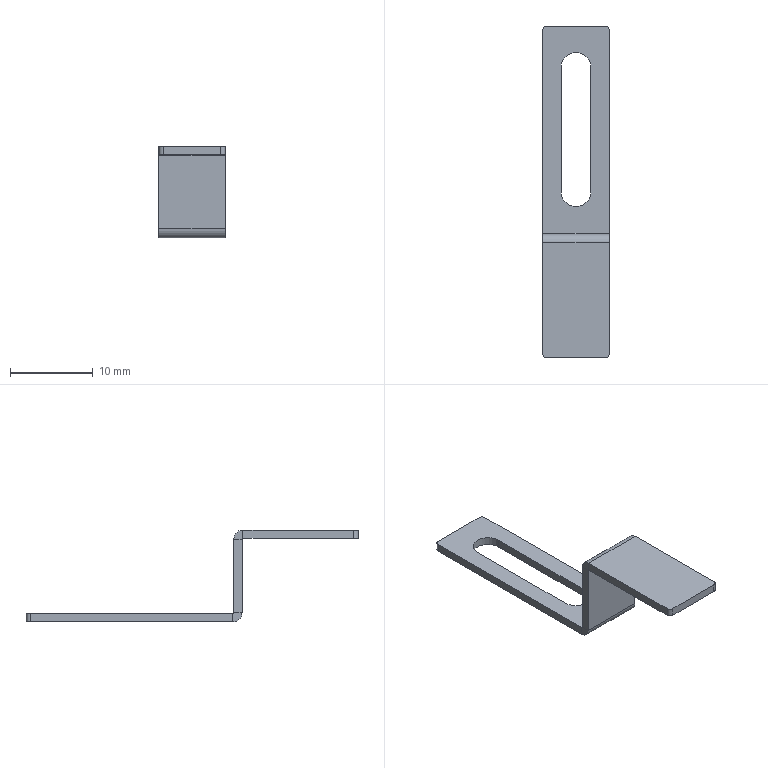Part | STEP file | Photoelectric sensor flag | 1 solid | 30 faces | box 8 x 40.1 x 11.1 mm | volume 333.086 mm3 | plane 20 | cylinder 10 | commonest cylinder face diameters 1 x4 0.2 x2 2.2 x2 3.6 x2